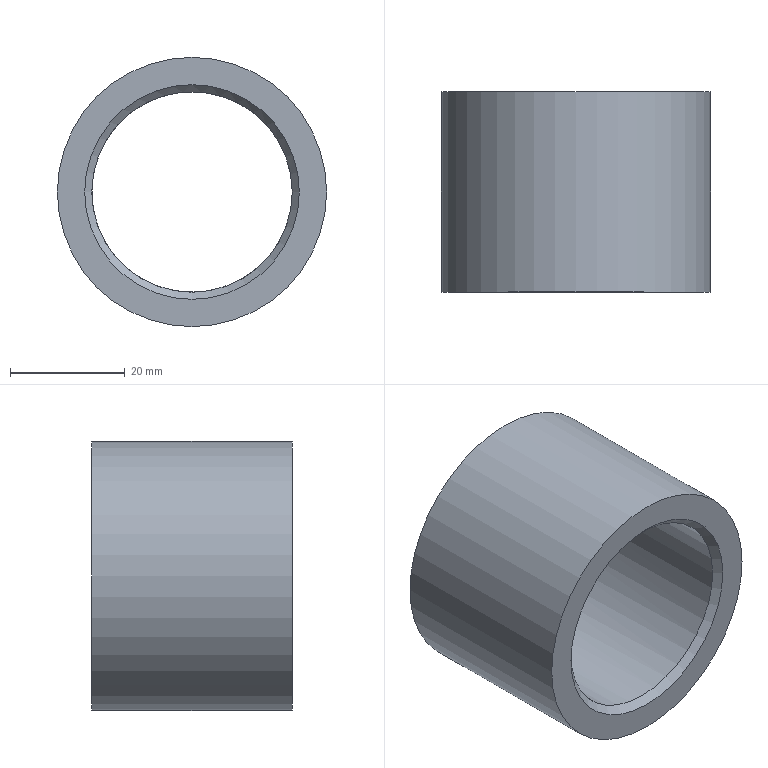Part | STEP file | GUIDE1_id270_x_t | 1 solid | 6 faces | box 47 x 35 x 47 mm | volume 26873 mm3 | cylinder 2 | cone 2 | plane 2 | commonest cylinder face diameters 35 x1 47 x1
STEP:
#1=CARTESIAN_POINT('',(-144.5,124.25,-235.));
#2=VERTEX_POINT('',#1);
#3=CARTESIAN_POINT('',(-162.,124.25,-235.));
#4=DIRECTION('',(0.,1.,0.));
#5=DIRECTION('',(1.,0.,0.));
#6=AXIS2_PLACEMENT_3D('',#3,#4,#5);
#7=CIRCLE('',#6,17.5);
#8=EDGE_CURVE('',#2,#2,#7,.T.);
#9=ORIENTED_EDGE('',*,*,#8,.T.);
#10=EDGE_LOOP('',(#9));
#11=FACE_BOUND('',#10,.T.);
#12=CARTESIAN_POINT('',(-179.5,91.75,-235.));
#13=VERTEX_POINT('',#12);
#14=CARTESIAN_POINT('',(-162.,91.75,-235.));
#15=DIRECTION('',(0.,-1.,0.));
#16=DIRECTION('',(-1.,0.,0.));
#17=AXIS2_PLACEMENT_3D('',#14,#15,#16);
#18=CIRCLE('',#17,17.5);
#19=EDGE_CURVE('',#13,#13,#18,.T.);
#20=ORIENTED_EDGE('',*,*,#19,.T.);
#21=EDGE_LOOP('',(#20));
#22=FACE_BOUND('',#21,.T.);
#23=CARTESIAN_POINT('',(-162.,88.75,-235.));
#24=DIRECTION('',(0.,-1.,0.));
#25=DIRECTION('',(0.,0.,-1.));
#26=AXIS2_PLACEMENT_3D('',#23,#24,#25);
#27=CYLINDRICAL_SURFACE('',#26,17.5);
#28=ADVANCED_FACE('',(#11,#22),#27,.F.);
#29=CARTESIAN_POINT('',(-162.,125.5,-216.25));
#30=VERTEX_POINT('',#29);
#31=CARTESIAN_POINT('',(-162.,125.5,-235.));
#32=DIRECTION('',(0.,1.,0.));
#33=DIRECTION('',(0.,0.,1.));
#34=AXIS2_PLACEMENT_3D('',#31,#32,#33);
#35=CIRCLE('',#34,18.75);
#36=EDGE_CURVE('',#30,#30,#35,.T.);
#37=ORIENTED_EDGE('',*,*,#36,.T.);
#38=EDGE_LOOP('',(#37));
#39=FACE_BOUND('',#38,.T.);
#40=ORIENTED_EDGE('',*,*,#8,.F.);
#41=EDGE_LOOP('',(#40));
#42=FACE_BOUND('',#41,.T.);
#43=CARTESIAN_POINT('',(-162.,125.5,-235.));
#44=DIRECTION('',(0.,1.,0.));
#45=DIRECTION('',(0.,0.,1.));
#46=AXIS2_PLACEMENT_3D('',#43,#44,#45);
#47=CONICAL_SURFACE('',#46,18.75,45.);
#48=ADVANCED_FACE('',(#39,#42),#47,.F.);
#49=ORIENTED_EDGE('',*,*,#19,.F.);
#50=EDGE_LOOP('',(#49));
#51=FACE_BOUND('',#50,.T.);
#52=CARTESIAN_POINT('',(-162.,90.5,-253.75));
#53=VERTEX_POINT('',#52);
#54=CARTESIAN_POINT('',(-162.,90.5,-235.));
#55=DIRECTION('',(0.,1.,0.));
#56=DIRECTION('',(0.,0.,-1.));
#57=AXIS2_PLACEMENT_3D('',#54,#55,#56);
#58=CIRCLE('',#57,18.75);
#59=EDGE_CURVE('',#53,#53,#58,.T.);
#60=ORIENTED_EDGE('',*,*,#59,.F.);
#61=EDGE_LOOP('',(#60));
#62=FACE_BOUND('',#61,.T.);
#63=CARTESIAN_POINT('',(-162.,90.5,-235.));
#64=DIRECTION('',(0.,-1.,0.));
#65=DIRECTION('',(0.,0.,-1.));
#66=AXIS2_PLACEMENT_3D('',#63,#64,#65);
#67=CONICAL_SURFACE('',#66,18.75,45.);
#68=ADVANCED_FACE('',(#51,#62),#67,.F.);
#69=ORIENTED_EDGE('',*,*,#36,.F.);
#70=EDGE_LOOP('',(#69));
#71=FACE_BOUND('',#70,.T.);
#72=CARTESIAN_POINT('',(-162.,125.5,-258.5));
#73=VERTEX_POINT('',#72);
#74=CARTESIAN_POINT('',(-162.,125.5,-235.));
#75=DIRECTION('',(0.,-1.,0.));
#76=DIRECTION('',(0.,0.,-1.));
#77=AXIS2_PLACEMENT_3D('',#74,#75,#76);
#78=CIRCLE('',#77,23.5);
#79=EDGE_CURVE('',#73,#73,#78,.T.);
#80=ORIENTED_EDGE('',*,*,#79,.F.);
#81=EDGE_LOOP('',(#80));
#82=FACE_BOUND('',#81,.T.);
#83=CARTESIAN_POINT('',(-162.,125.5,-235.));
#84=DIRECTION('',(0.,-1.,0.));
#85=DIRECTION('',(0.,0.,-1.));
#86=AXIS2_PLACEMENT_3D('',#83,#84,#85);
#87=PLANE('',#86);
#88=ADVANCED_FACE('',(#71,#82),#87,.F.);
#89=ORIENTED_EDGE('',*,*,#59,.T.);
#90=EDGE_LOOP('',(#89));
#91=FACE_BOUND('',#90,.T.);
#92=CARTESIAN_POINT('',(-162.,90.5,-258.5));
#93=VERTEX_POINT('',#92);
#94=CARTESIAN_POINT('',(-162.,90.5,-235.));
#95=DIRECTION('',(0.,1.,0.));
#96=DIRECTION('',(0.,0.,-1.));
#97=AXIS2_PLACEMENT_3D('',#94,#95,#96);
#98=CIRCLE('',#97,23.5);
#99=EDGE_CURVE('',#93,#93,#98,.T.);
#100=ORIENTED_EDGE('',*,*,#99,.F.);
#101=EDGE_LOOP('',(#100));
#102=FACE_BOUND('',#101,.T.);
#103=CARTESIAN_POINT('',(-162.,90.5,-235.));
#104=DIRECTION('',(0.,-1.,0.));
#105=DIRECTION('',(0.,0.,-1.));
#106=AXIS2_PLACEMENT_3D('',#103,#104,#105);
#107=PLANE('',#106);
#108=ADVANCED_FACE('',(#91,#102),#107,.T.);
#109=ORIENTED_EDGE('',*,*,#99,.T.);
#110=EDGE_LOOP('',(#109));
#111=FACE_BOUND('',#110,.T.);
#112=ORIENTED_EDGE('',*,*,#79,.T.);
#113=EDGE_LOOP('',(#112));
#114=FACE_BOUND('',#113,.T.);
#115=CARTESIAN_POINT('',(-162.,88.75,-235.));
#116=DIRECTION('',(0.,-1.,0.));
#117=DIRECTION('',(0.,0.,-1.));
#118=AXIS2_PLACEMENT_3D('',#115,#116,#117);
#119=CYLINDRICAL_SURFACE('',#118,23.5);
#120=ADVANCED_FACE('',(#111,#114),#119,.T.);
#121=CLOSED_SHELL('',(#28,#48,#68,#88,#108,#120));
#122=MANIFOLD_SOLID_BREP('',#121);
#123=(LENGTH_UNIT()NAMED_UNIT(*)SI_UNIT(.MILLI.,.METRE.));
#124=UNCERTAINTY_MEASURE_WITH_UNIT(LENGTH_MEASURE(0.00002),#123,'','');
#125=(NAMED_UNIT(*)PLANE_ANGLE_UNIT()SI_UNIT($,.RADIAN.));
#126=PLANE_ANGLE_MEASURE_WITH_UNIT(PLANE_ANGLE_MEASURE(0.01745),#125);
#127=DIMENSIONAL_EXPONENTS(0.,0.,0.,0.,0.,0.,0.);
#128=(CONVERSION_BASED_UNIT('DEGREE',#126)NAMED_UNIT(#127)PLANE_ANGLE_UNIT());
#129=(NAMED_UNIT(*)SI_UNIT($,.STERADIAN.)SOLID_ANGLE_UNIT());
#130=(GEOMETRIC_REPRESENTATION_CONTEXT(3)GLOBAL_UNCERTAINTY_ASSIGNED_CONTEXT((#124))GLOBAL_UNIT_ASSIGNED_CONTEXT((#123,#128,#129))REPRESENTATION_CONTEXT('',''));
#131=ADVANCED_BREP_SHAPE_REPRESENTATION('',(#122),#130);